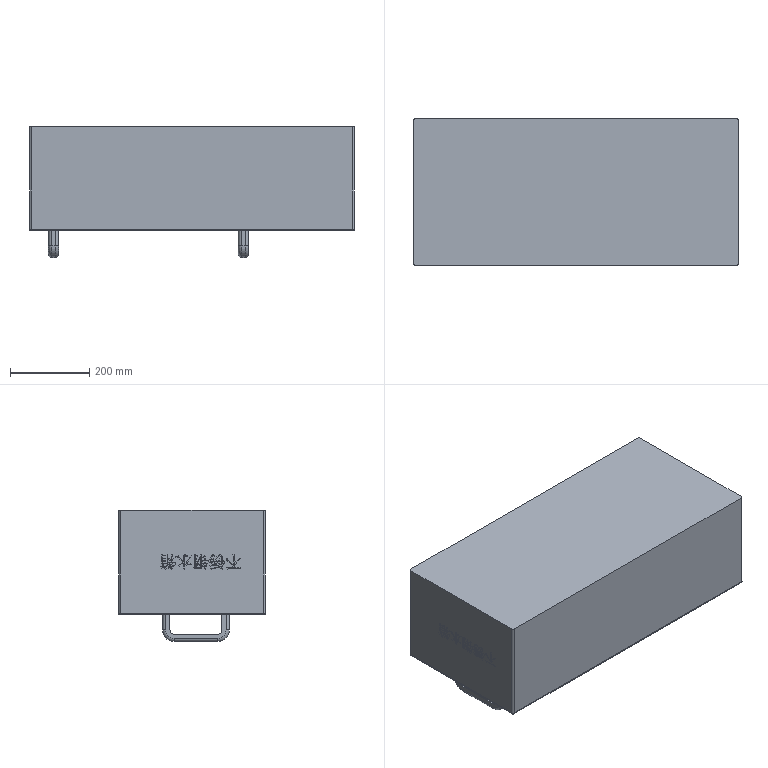Part | STEP file | PN_0004 Stainless steel water tank | 2 solids | 343 faces | box 820 x 370 x 331.29 mm | volume 9708465 mm3 | plane 226 | spline 81 | cylinder 28 | torus 8 | commonest cylinder face diameters 16 x12 6 x4 10 x4 21.42 x4 58.58 x4